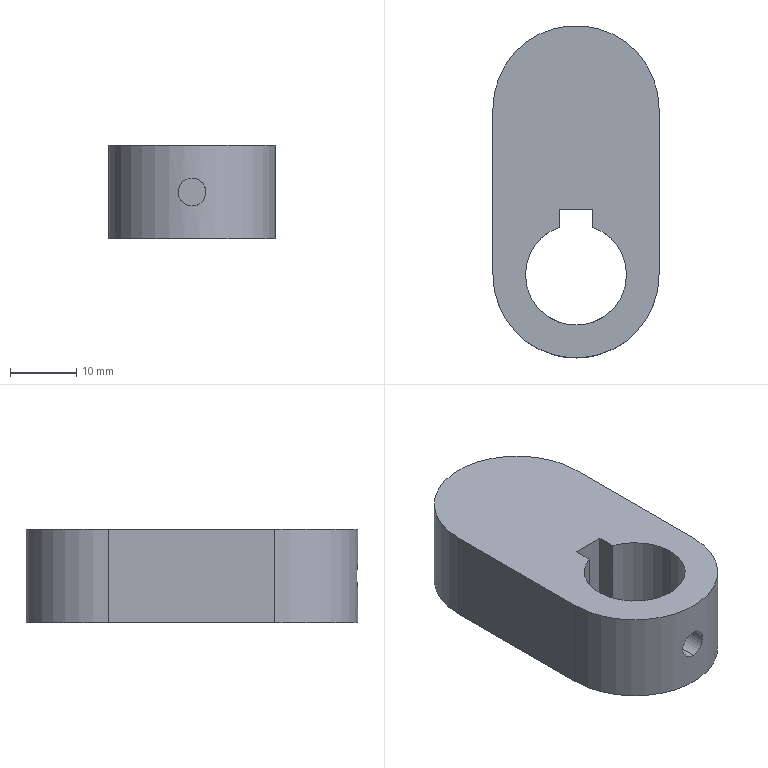Part | SolidWorks | features Extrusion 1, HoleWzd 1 | 1 solid | 14 faces | box 25 x 50 x 14 mm | volume 12843 mm3 | cylinder 7 | plane 7 | commonest cylinder face diameters 15.2 x3 4.2 x2 25 x2
STEP:
#1=CARTESIAN_POINT('',(0.,-12.5,4.9));
#2=VERTEX_POINT('',#1);
#3=CARTESIAN_POINT('',(0.,-12.5,9.1));
#4=VERTEX_POINT('',#3);
#5=CARTESIAN_POINT('',(0.,-12.5,4.9));
#6=CARTESIAN_POINT('',(-0.2743,-12.5,4.9));
#7=CARTESIAN_POINT('',(-0.5511,-12.49,4.955));
#8=CARTESIAN_POINT('',(-0.9302,-12.466,5.112));
#9=CARTESIAN_POINT('',(-1.053,-12.456,5.178));
#10=CARTESIAN_POINT('',(-1.282,-12.435,5.331));
#11=CARTESIAN_POINT('',(-1.387,-12.423,5.417));
#12=CARTESIAN_POINT('',(-1.581,-12.4,5.611));
#13=CARTESIAN_POINT('',(-1.669,-12.388,5.719));
#14=CARTESIAN_POINT('',(-1.822,-12.367,5.946));
#15=CARTESIAN_POINT('',(-1.886,-12.357,6.067));
#16=CARTESIAN_POINT('',(-1.992,-12.34,6.321));
#17=CARTESIAN_POINT('',(-2.032,-12.334,6.454));
#18=CARTESIAN_POINT('',(-2.086,-12.325,6.723));
#19=CARTESIAN_POINT('',(-2.1,-12.322,6.86));
#20=CARTESIAN_POINT('',(-2.1,-12.322,7.137));
#21=CARTESIAN_POINT('',(-2.087,-12.325,7.274));
#22=CARTESIAN_POINT('',(-2.033,-12.334,7.543));
#23=CARTESIAN_POINT('',(-1.993,-12.34,7.677));
#24=CARTESIAN_POINT('',(-1.888,-12.357,7.931));
#25=CARTESIAN_POINT('',(-1.823,-12.367,8.051));
#26=CARTESIAN_POINT('',(-1.671,-12.388,8.28));
#27=CARTESIAN_POINT('',(-1.582,-12.4,8.387));
#28=CARTESIAN_POINT('',(-1.293,-12.434,8.677));
#29=CARTESIAN_POINT('',(-1.059,-12.458,8.834));
#30=CARTESIAN_POINT('',(-0.6803,-12.482,8.991));
#31=CARTESIAN_POINT('',(-0.5475,-12.489,9.032));
#32=CARTESIAN_POINT('',(-0.2763,-12.498,9.086));
#33=CARTESIAN_POINT('',(-0.139,-12.5,9.1));
#34=CARTESIAN_POINT('',(0.,-12.5,9.1));
#35=B_SPLINE_CURVE_WITH_KNOTS('',3,(#5,#6,#7,#8,#9,#10,#11,#12,#13,#14,#15,#16,#17,#18,#19,#20,#21,#22,#23,#24,#25,#26,#27,#28,#29,#30,#31,#32,#33,#34),.UNSPECIFIED.,.F.,.F.,(4,2,2,2,2,2,2,2,2,2,2,2,2,2,4),(0.006577,0.007399,0.00781,0.008221,0.008632,0.009043,0.009454,0.009865,0.01028,0.01069,0.0111,0.01151,0.01233,0.01274,0.01315),.UNSPECIFIED.);
#36=EDGE_CURVE('',#2,#4,#35,.T.);
#37=ORIENTED_EDGE('',*,*,#36,.F.);
#38=CARTESIAN_POINT('',(0.,-7.6,4.9));
#39=VERTEX_POINT('',#38);
#40=CARTESIAN_POINT('',(0.,0.,4.9));
#41=DIRECTION('',(0.,1.,0.));
#42=VECTOR('',#41,1000.);
#43=LINE('',#40,#42);
#44=EDGE_CURVE('',#2,#39,#43,.T.);
#45=ORIENTED_EDGE('',*,*,#44,.T.);
#46=CARTESIAN_POINT('',(0.,-7.6,9.1));
#47=VERTEX_POINT('',#46);
#48=CARTESIAN_POINT('',(0.,-7.6,4.9));
#49=CARTESIAN_POINT('',(-0.2749,-7.6,4.9));
#50=CARTESIAN_POINT('',(-0.5524,-7.584,4.956));
#51=CARTESIAN_POINT('',(-0.932,-7.544,5.113));
#52=CARTESIAN_POINT('',(-1.055,-7.527,5.179));
#53=CARTESIAN_POINT('',(-1.282,-7.492,5.331));
#54=CARTESIAN_POINT('',(-1.388,-7.473,5.418));
#55=CARTESIAN_POINT('',(-1.581,-7.434,5.611));
#56=CARTESIAN_POINT('',(-1.669,-7.415,5.719));
#57=CARTESIAN_POINT('',(-1.821,-7.379,5.945));
#58=CARTESIAN_POINT('',(-1.886,-7.363,6.066));
#59=CARTESIAN_POINT('',(-1.992,-7.334,6.321));
#60=CARTESIAN_POINT('',(-2.032,-7.323,6.453));
#61=CARTESIAN_POINT('',(-2.086,-7.308,6.722));
#62=CARTESIAN_POINT('',(-2.1,-7.304,6.861));
#63=CARTESIAN_POINT('',(-2.1,-7.304,7.138));
#64=CARTESIAN_POINT('',(-2.086,-7.308,7.275));
#65=CARTESIAN_POINT('',(-2.033,-7.323,7.545));
#66=CARTESIAN_POINT('',(-1.992,-7.335,7.679));
#67=CARTESIAN_POINT('',(-1.834,-7.376,8.059));
#68=CARTESIAN_POINT('',(-1.678,-7.415,8.292));
#69=CARTESIAN_POINT('',(-1.389,-7.473,8.581));
#70=CARTESIAN_POINT('',(-1.283,-7.492,8.668));
#71=CARTESIAN_POINT('',(-1.054,-7.527,8.821));
#72=CARTESIAN_POINT('',(-0.9341,-7.543,8.886));
#73=CARTESIAN_POINT('',(-0.6811,-7.57,8.991));
#74=CARTESIAN_POINT('',(-0.5471,-7.581,9.032));
#75=CARTESIAN_POINT('',(-0.2767,-7.596,9.086));
#76=CARTESIAN_POINT('',(-0.1394,-7.6,9.1));
#77=CARTESIAN_POINT('',(0.,-7.6,9.1));
#78=B_SPLINE_CURVE_WITH_KNOTS('',3,(#48,#49,#50,#51,#52,#53,#54,#55,#56,#57,#58,#59,#60,#61,#62,#63,#64,#65,#66,#67,#68,#69,#70,#71,#72,#73,#74,#75,#76,#77),.UNSPECIFIED.,.F.,.F.,(4,2,2,2,2,2,2,2,2,2,2,2,2,2,4),(0.006598,0.007422,0.007835,0.008247,0.008659,0.009071,0.009484,0.009896,0.01031,0.01072,0.01154,0.01196,0.01237,0.01278,0.01319),.UNSPECIFIED.);
#79=EDGE_CURVE('',#39,#47,#78,.T.);
#80=ORIENTED_EDGE('',*,*,#79,.T.);
#81=CARTESIAN_POINT('',(0.,0.,9.1));
#82=DIRECTION('',(0.,1.,0.));
#83=VECTOR('',#82,1000.);
#84=LINE('',#81,#83);
#85=EDGE_CURVE('',#4,#47,#84,.T.);
#86=ORIENTED_EDGE('',*,*,#85,.F.);
#87=EDGE_LOOP('',(#37,#45,#80,#86));
#88=FACE_OUTER_BOUND('',#87,.T.);
#89=CARTESIAN_POINT('',(0.,0.,7.));
#90=DIRECTION('',(0.,1.,0.));
#91=DIRECTION('',(0.,0.,1.));
#92=AXIS2_PLACEMENT_3D('',#89,#90,#91);
#93=CYLINDRICAL_SURFACE('',#92,2.1);
#94=ADVANCED_FACE('',(#88),#93,.F.);
#95=CARTESIAN_POINT('',(0.,-7.6,9.1));
#96=CARTESIAN_POINT('',(0.1395,-7.6,9.1));
#97=CARTESIAN_POINT('',(0.2765,-7.596,9.086));
#98=CARTESIAN_POINT('',(0.5459,-7.582,9.032));
#99=CARTESIAN_POINT('',(0.6796,-7.571,8.992));
#100=CARTESIAN_POINT('',(0.9337,-7.544,8.886));
#101=CARTESIAN_POINT('',(1.054,-7.527,8.821));
#102=CARTESIAN_POINT('',(1.282,-7.492,8.669));
#103=CARTESIAN_POINT('',(1.389,-7.473,8.581));
#104=CARTESIAN_POINT('',(1.678,-7.415,8.292));
#105=CARTESIAN_POINT('',(1.834,-7.376,8.058));
#106=CARTESIAN_POINT('',(1.992,-7.335,7.68));
#107=CARTESIAN_POINT('',(2.032,-7.323,7.547));
#108=CARTESIAN_POINT('',(2.086,-7.308,7.275));
#109=CARTESIAN_POINT('',(2.1,-7.304,7.139));
#110=CARTESIAN_POINT('',(2.1,-7.304,6.863));
#111=CARTESIAN_POINT('',(2.086,-7.308,6.723));
#112=CARTESIAN_POINT('',(2.032,-7.323,6.453));
#113=CARTESIAN_POINT('',(1.992,-7.334,6.322));
#114=CARTESIAN_POINT('',(1.833,-7.376,5.939));
#115=CARTESIAN_POINT('',(1.679,-7.415,5.709));
#116=CARTESIAN_POINT('',(1.387,-7.473,5.418));
#117=CARTESIAN_POINT('',(1.282,-7.492,5.331));
#118=CARTESIAN_POINT('',(1.055,-7.527,5.179));
#119=CARTESIAN_POINT('',(0.9321,-7.544,5.113));
#120=CARTESIAN_POINT('',(0.6787,-7.571,5.008));
#121=CARTESIAN_POINT('',(0.5477,-7.581,4.968));
#122=CARTESIAN_POINT('',(0.2769,-7.596,4.914));
#123=CARTESIAN_POINT('',(0.1375,-7.6,4.9));
#124=CARTESIAN_POINT('',(0.,-7.6,4.9));
#125=B_SPLINE_CURVE_WITH_KNOTS('',3,(#95,#96,#97,#98,#99,#100,#101,#102,#103,#104,#105,#106,#107,#108,#109,#110,#111,#112,#113,#114,#115,#116,#117,#118,#119,#120,#121,#122,#123,#124),.UNSPECIFIED.,.F.,.F.,(4,2,2,2,2,2,2,2,2,2,2,2,2,2,4),(0.,0.0004124,0.0008247,0.001237,0.001649,0.002474,0.002887,0.003299,0.003711,0.004124,0.004948,0.005361,0.005773,0.006185,0.006598),.UNSPECIFIED.);
#126=EDGE_CURVE('',#47,#39,#125,.T.);
#127=ORIENTED_EDGE('',*,*,#126,.F.);
#128=ORIENTED_EDGE('',*,*,#79,.F.);
#129=EDGE_LOOP('',(#127,#128));
#130=FACE_BOUND('',#129,.T.);
#131=CARTESIAN_POINT('',(-7.6,0.,14.));
#132=VERTEX_POINT('',#131);
#133=CARTESIAN_POINT('',(7.6,0.,14.));
#134=VERTEX_POINT('',#133);
#135=CARTESIAN_POINT('',(0.,0.,14.));
#136=DIRECTION('',(0.,0.,1.));
#137=DIRECTION('',(1.,0.,0.));
#138=AXIS2_PLACEMENT_3D('',#135,#136,#137);
#139=CIRCLE('',#138,7.6);
#140=EDGE_CURVE('',#132,#134,#139,.T.);
#141=ORIENTED_EDGE('',*,*,#140,.T.);
#142=CARTESIAN_POINT('',(7.6,0.,0.));
#143=VERTEX_POINT('',#142);
#144=CARTESIAN_POINT('',(7.6,0.,14.));
#145=DIRECTION('',(0.,0.,-1.));
#146=VECTOR('',#145,1000.);
#147=LINE('',#144,#146);
#148=EDGE_CURVE('',#134,#143,#147,.T.);
#149=ORIENTED_EDGE('',*,*,#148,.T.);
#150=CARTESIAN_POINT('',(-7.6,0.,0.));
#151=VERTEX_POINT('',#150);
#152=CARTESIAN_POINT('',(0.,0.,0.));
#153=DIRECTION('',(0.,0.,1.));
#154=DIRECTION('',(1.,0.,0.));
#155=AXIS2_PLACEMENT_3D('',#152,#153,#154);
#156=CIRCLE('',#155,7.6);
#157=EDGE_CURVE('',#151,#143,#156,.T.);
#158=ORIENTED_EDGE('',*,*,#157,.F.);
#159=CARTESIAN_POINT('',(-7.6,0.,14.));
#160=DIRECTION('',(0.,0.,-1.));
#161=VECTOR('',#160,1000.);
#162=LINE('',#159,#161);
#163=EDGE_CURVE('',#132,#151,#162,.T.);
#164=ORIENTED_EDGE('',*,*,#163,.F.);
#165=EDGE_LOOP('',(#141,#149,#158,#164));
#166=FACE_OUTER_BOUND('',#165,.T.);
#167=CARTESIAN_POINT('',(0.,0.,14.));
#168=DIRECTION('',(0.,0.,-1.));
#169=DIRECTION('',(-1.,0.,0.));
#170=AXIS2_PLACEMENT_3D('',#167,#168,#169);
#171=CYLINDRICAL_SURFACE('',#170,7.6);
#172=ADVANCED_FACE('',(#130,#166),#171,.F.);
#173=CARTESIAN_POINT('',(-2.5,7.177,14.));
#174=VERTEX_POINT('',#173);
#175=CARTESIAN_POINT('',(0.,0.,14.));
#176=DIRECTION('',(0.,0.,1.));
#177=DIRECTION('',(1.,0.,0.));
#178=AXIS2_PLACEMENT_3D('',#175,#176,#177);
#179=CIRCLE('',#178,7.6);
#180=EDGE_CURVE('',#174,#132,#179,.T.);
#181=ORIENTED_EDGE('',*,*,#180,.T.);
#182=ORIENTED_EDGE('',*,*,#163,.T.);
#183=CARTESIAN_POINT('',(-2.5,7.177,0.));
#184=VERTEX_POINT('',#183);
#185=CARTESIAN_POINT('',(0.,0.,0.));
#186=DIRECTION('',(0.,0.,1.));
#187=DIRECTION('',(1.,0.,0.));
#188=AXIS2_PLACEMENT_3D('',#185,#186,#187);
#189=CIRCLE('',#188,7.6);
#190=EDGE_CURVE('',#184,#151,#189,.T.);
#191=ORIENTED_EDGE('',*,*,#190,.F.);
#192=CARTESIAN_POINT('',(-2.5,7.177,14.));
#193=DIRECTION('',(0.,0.,-1.));
#194=VECTOR('',#193,1000.);
#195=LINE('',#192,#194);
#196=EDGE_CURVE('',#174,#184,#195,.T.);
#197=ORIENTED_EDGE('',*,*,#196,.F.);
#198=EDGE_LOOP('',(#181,#182,#191,#197));
#199=FACE_OUTER_BOUND('',#198,.T.);
#200=CARTESIAN_POINT('',(0.,0.,14.));
#201=DIRECTION('',(0.,0.,-1.));
#202=DIRECTION('',(-1.,0.,0.));
#203=AXIS2_PLACEMENT_3D('',#200,#201,#202);
#204=CYLINDRICAL_SURFACE('',#203,7.6);
#205=ADVANCED_FACE('',(#199),#204,.F.);
#206=CARTESIAN_POINT('',(12.5,0.,0.));
#207=VERTEX_POINT('',#206);
#208=CARTESIAN_POINT('',(12.5,25.,0.));
#209=VERTEX_POINT('',#208);
#210=CARTESIAN_POINT('',(12.5,0.,0.));
#211=DIRECTION('',(0.,1.,0.));
#212=VECTOR('',#211,1000.);
#213=LINE('',#210,#212);
#214=EDGE_CURVE('',#207,#209,#213,.T.);
#215=ORIENTED_EDGE('',*,*,#214,.T.);
#216=CARTESIAN_POINT('',(12.5,25.,14.));
#217=VERTEX_POINT('',#216);
#218=CARTESIAN_POINT('',(12.5,25.,14.));
#219=DIRECTION('',(0.,0.,-1.));
#220=VECTOR('',#219,1000.);
#221=LINE('',#218,#220);
#222=EDGE_CURVE('',#217,#209,#221,.T.);
#223=ORIENTED_EDGE('',*,*,#222,.F.);
#224=CARTESIAN_POINT('',(12.5,0.,14.));
#225=VERTEX_POINT('',#224);
#226=CARTESIAN_POINT('',(12.5,0.,14.));
#227=DIRECTION('',(0.,1.,0.));
#228=VECTOR('',#227,1000.);
#229=LINE('',#226,#228);
#230=EDGE_CURVE('',#225,#217,#229,.T.);
#231=ORIENTED_EDGE('',*,*,#230,.F.);
#232=CARTESIAN_POINT('',(12.5,0.,14.));
#233=DIRECTION('',(0.,0.,-1.));
#234=VECTOR('',#233,1000.);
#235=LINE('',#232,#234);
#236=EDGE_CURVE('',#225,#207,#235,.T.);
#237=ORIENTED_EDGE('',*,*,#236,.T.);
#238=EDGE_LOOP('',(#215,#223,#231,#237));
#239=FACE_OUTER_BOUND('',#238,.T.);
#240=CARTESIAN_POINT('',(12.5,0.,14.));
#241=DIRECTION('',(-1.,0.,0.));
#242=DIRECTION('',(0.,0.,1.));
#243=AXIS2_PLACEMENT_3D('',#240,#241,#242);
#244=PLANE('',#243);
#245=ADVANCED_FACE('',(#239),#244,.F.);
#246=CARTESIAN_POINT('',(-12.5,25.,0.));
#247=VERTEX_POINT('',#246);
#248=CARTESIAN_POINT('',(0.,25.,0.));
#249=DIRECTION('',(0.,0.,1.));
#250=DIRECTION('',(1.,0.,0.));
#251=AXIS2_PLACEMENT_3D('',#248,#249,#250);
#252=CIRCLE('',#251,12.5);
#253=EDGE_CURVE('',#209,#247,#252,.T.);
#254=ORIENTED_EDGE('',*,*,#253,.T.);
#255=CARTESIAN_POINT('',(-12.5,25.,14.));
#256=VERTEX_POINT('',#255);
#257=CARTESIAN_POINT('',(-12.5,25.,14.));
#258=DIRECTION('',(0.,0.,-1.));
#259=VECTOR('',#258,1000.);
#260=LINE('',#257,#259);
#261=EDGE_CURVE('',#256,#247,#260,.T.);
#262=ORIENTED_EDGE('',*,*,#261,.F.);
#263=CARTESIAN_POINT('',(0.,25.,14.));
#264=DIRECTION('',(0.,0.,1.));
#265=DIRECTION('',(1.,0.,0.));
#266=AXIS2_PLACEMENT_3D('',#263,#264,#265);
#267=CIRCLE('',#266,12.5);
#268=EDGE_CURVE('',#217,#256,#267,.T.);
#269=ORIENTED_EDGE('',*,*,#268,.F.);
#270=ORIENTED_EDGE('',*,*,#222,.T.);
#271=EDGE_LOOP('',(#254,#262,#269,#270));
#272=FACE_OUTER_BOUND('',#271,.T.);
#273=CARTESIAN_POINT('',(0.,25.,14.));
#274=DIRECTION('',(0.,0.,-1.));
#275=DIRECTION('',(-1.,0.,0.));
#276=AXIS2_PLACEMENT_3D('',#273,#274,#275);
#277=CYLINDRICAL_SURFACE('',#276,12.5);
#278=ADVANCED_FACE('',(#272),#277,.T.);
#279=CARTESIAN_POINT('',(-12.5,0.,0.));
#280=VERTEX_POINT('',#279);
#281=CARTESIAN_POINT('',(-12.5,0.,0.));
#282=DIRECTION('',(0.,1.,0.));
#283=VECTOR('',#282,1000.);
#284=LINE('',#281,#283);
#285=EDGE_CURVE('',#280,#247,#284,.T.);
#286=ORIENTED_EDGE('',*,*,#285,.F.);
#287=CARTESIAN_POINT('',(-12.5,0.,14.));
#288=VERTEX_POINT('',#287);
#289=CARTESIAN_POINT('',(-12.5,0.,14.));
#290=DIRECTION('',(0.,0.,-1.));
#291=VECTOR('',#290,1000.);
#292=LINE('',#289,#291);
#293=EDGE_CURVE('',#288,#280,#292,.T.);
#294=ORIENTED_EDGE('',*,*,#293,.F.);
#295=CARTESIAN_POINT('',(-12.5,0.,14.));
#296=DIRECTION('',(0.,1.,0.));
#297=VECTOR('',#296,1000.);
#298=LINE('',#295,#297);
#299=EDGE_CURVE('',#288,#256,#298,.T.);
#300=ORIENTED_EDGE('',*,*,#299,.T.);
#301=ORIENTED_EDGE('',*,*,#261,.T.);
#302=EDGE_LOOP('',(#286,#294,#300,#301));
#303=FACE_OUTER_BOUND('',#302,.T.);
#304=CARTESIAN_POINT('',(-12.5,0.,14.));
#305=DIRECTION('',(-1.,0.,0.));
#306=DIRECTION('',(0.,0.,1.));
#307=AXIS2_PLACEMENT_3D('',#304,#305,#306);
#308=PLANE('',#307);
#309=ADVANCED_FACE('',(#303),#308,.T.);
#310=ORIENTED_EDGE('',*,*,#148,.F.);
#311=CARTESIAN_POINT('',(2.5,7.177,14.));
#312=VERTEX_POINT('',#311);
#313=CARTESIAN_POINT('',(0.,0.,14.));
#314=DIRECTION('',(0.,0.,1.));
#315=DIRECTION('',(1.,0.,0.));
#316=AXIS2_PLACEMENT_3D('',#313,#314,#315);
#317=CIRCLE('',#316,7.6);
#318=EDGE_CURVE('',#134,#312,#317,.T.);
#319=ORIENTED_EDGE('',*,*,#318,.T.);
#320=CARTESIAN_POINT('',(2.5,7.177,0.));
#321=VERTEX_POINT('',#320);
#322=CARTESIAN_POINT('',(2.5,7.177,14.));
#323=DIRECTION('',(0.,0.,-1.));
#324=VECTOR('',#323,1000.);
#325=LINE('',#322,#324);
#326=EDGE_CURVE('',#312,#321,#325,.T.);
#327=ORIENTED_EDGE('',*,*,#326,.T.);
#328=CARTESIAN_POINT('',(0.,0.,0.));
#329=DIRECTION('',(0.,0.,1.));
#330=DIRECTION('',(1.,0.,0.));
#331=AXIS2_PLACEMENT_3D('',#328,#329,#330);
#332=CIRCLE('',#331,7.6);
#333=EDGE_CURVE('',#143,#321,#332,.T.);
#334=ORIENTED_EDGE('',*,*,#333,.F.);
#335=EDGE_LOOP('',(#310,#319,#327,#334));
#336=FACE_OUTER_BOUND('',#335,.T.);
#337=CARTESIAN_POINT('',(0.,0.,14.));
#338=DIRECTION('',(0.,0.,-1.));
#339=DIRECTION('',(-1.,0.,0.));
#340=AXIS2_PLACEMENT_3D('',#337,#338,#339);
#341=CYLINDRICAL_SURFACE('',#340,7.6);
#342=ADVANCED_FACE('',(#336),#341,.F.);
#343=CARTESIAN_POINT('',(-2.5,9.9,0.));
#344=VERTEX_POINT('',#343);
#345=CARTESIAN_POINT('',(-2.5,0.,0.));
#346=DIRECTION('',(0.,1.,0.));
#347=VECTOR('',#346,1000.);
#348=LINE('',#345,#347);
#349=EDGE_CURVE('',#184,#344,#348,.T.);
#350=ORIENTED_EDGE('',*,*,#349,.T.);
#351=CARTESIAN_POINT('',(-2.5,9.9,14.));
#352=VERTEX_POINT('',#351);
#353=CARTESIAN_POINT('',(-2.5,9.9,14.));
#354=DIRECTION('',(0.,0.,-1.));
#355=VECTOR('',#354,1000.);
#356=LINE('',#353,#355);
#357=EDGE_CURVE('',#352,#344,#356,.T.);
#358=ORIENTED_EDGE('',*,*,#357,.F.);
#359=CARTESIAN_POINT('',(-2.5,0.,14.));
#360=DIRECTION('',(0.,1.,0.));
#361=VECTOR('',#360,1000.);
#362=LINE('',#359,#361);
#363=EDGE_CURVE('',#174,#352,#362,.T.);
#364=ORIENTED_EDGE('',*,*,#363,.F.);
#365=ORIENTED_EDGE('',*,*,#196,.T.);
#366=EDGE_LOOP('',(#350,#358,#364,#365));
#367=FACE_OUTER_BOUND('',#366,.T.);
#368=CARTESIAN_POINT('',(-2.5,0.,14.));
#369=DIRECTION('',(-1.,0.,0.));
#370=DIRECTION('',(0.,0.,1.));
#371=AXIS2_PLACEMENT_3D('',#368,#369,#370);
#372=PLANE('',#371);
#373=ADVANCED_FACE('',(#367),#372,.F.);
#374=CARTESIAN_POINT('',(2.5,9.9,0.));
#375=VERTEX_POINT('',#374);
#376=CARTESIAN_POINT('',(0.,9.9,0.));
#377=DIRECTION('',(-1.,0.,0.));
#378=VECTOR('',#377,1000.);
#379=LINE('',#376,#378);
#380=EDGE_CURVE('',#375,#344,#379,.T.);
#381=ORIENTED_EDGE('',*,*,#380,.F.);
#382=CARTESIAN_POINT('',(2.5,9.9,14.));
#383=VERTEX_POINT('',#382);
#384=CARTESIAN_POINT('',(2.5,9.9,14.));
#385=DIRECTION('',(0.,0.,-1.));
#386=VECTOR('',#385,1000.);
#387=LINE('',#384,#386);
#388=EDGE_CURVE('',#383,#375,#387,.T.);
#389=ORIENTED_EDGE('',*,*,#388,.F.);
#390=CARTESIAN_POINT('',(0.,9.9,14.));
#391=DIRECTION('',(-1.,0.,0.));
#392=VECTOR('',#391,1000.);
#393=LINE('',#390,#392);
#394=EDGE_CURVE('',#383,#352,#393,.T.);
#395=ORIENTED_EDGE('',*,*,#394,.T.);
#396=ORIENTED_EDGE('',*,*,#357,.T.);
#397=EDGE_LOOP('',(#381,#389,#395,#396));
#398=FACE_OUTER_BOUND('',#397,.T.);
#399=CARTESIAN_POINT('',(0.,9.9,14.));
#400=DIRECTION('',(0.,-1.,0.));
#401=DIRECTION('',(0.,0.,-1.));
#402=AXIS2_PLACEMENT_3D('',#399,#400,#401);
#403=PLANE('',#402);
#404=ADVANCED_FACE('',(#398),#403,.T.);
#405=CARTESIAN_POINT('',(2.5,0.,0.));
#406=DIRECTION('',(0.,1.,0.));
#407=VECTOR('',#406,1000.);
#408=LINE('',#405,#407);
#409=EDGE_CURVE('',#321,#375,#408,.T.);
#410=ORIENTED_EDGE('',*,*,#409,.F.);
#411=ORIENTED_EDGE('',*,*,#326,.F.);
#412=CARTESIAN_POINT('',(2.5,0.,14.));
#413=DIRECTION('',(0.,1.,0.));
#414=VECTOR('',#413,1000.);
#415=LINE('',#412,#414);
#416=EDGE_CURVE('',#312,#383,#415,.T.);
#417=ORIENTED_EDGE('',*,*,#416,.T.);
#418=ORIENTED_EDGE('',*,*,#388,.T.);
#419=EDGE_LOOP('',(#410,#411,#417,#418));
#420=FACE_OUTER_BOUND('',#419,.T.);
#421=CARTESIAN_POINT('',(2.5,0.,14.));
#422=DIRECTION('',(-1.,0.,0.));
#423=DIRECTION('',(0.,0.,1.));
#424=AXIS2_PLACEMENT_3D('',#421,#422,#423);
#425=PLANE('',#424);
#426=ADVANCED_FACE('',(#420),#425,.T.);
#427=CARTESIAN_POINT('',(0.,-12.5,9.1));
#428=CARTESIAN_POINT('',(0.139,-12.5,9.1));
#429=CARTESIAN_POINT('',(0.2757,-12.498,9.086));
#430=CARTESIAN_POINT('',(0.5444,-12.489,9.033));
#431=CARTESIAN_POINT('',(0.6779,-12.482,8.992));
#432=CARTESIAN_POINT('',(0.9322,-12.466,8.887));
#433=CARTESIAN_POINT('',(1.053,-12.456,8.822));
#434=CARTESIAN_POINT('',(1.281,-12.435,8.67));
#435=CARTESIAN_POINT('',(1.389,-12.423,8.581));
#436=CARTESIAN_POINT('',(1.679,-12.388,8.291));
#437=CARTESIAN_POINT('',(1.835,-12.365,8.057));
#438=CARTESIAN_POINT('',(2.045,-12.332,7.552));
#439=CARTESIAN_POINT('',(2.1,-12.322,7.275));
#440=CARTESIAN_POINT('',(2.1,-12.322,6.864));
#441=CARTESIAN_POINT('',(2.086,-12.325,6.724));
#442=CARTESIAN_POINT('',(2.033,-12.334,6.455));
#443=CARTESIAN_POINT('',(1.993,-12.34,6.324));
#444=CARTESIAN_POINT('',(1.887,-12.357,6.069));
#445=CARTESIAN_POINT('',(1.822,-12.367,5.946));
#446=CARTESIAN_POINT('',(1.67,-12.388,5.719));
#447=CARTESIAN_POINT('',(1.583,-12.4,5.613));
#448=CARTESIAN_POINT('',(1.387,-12.423,5.417));
#449=CARTESIAN_POINT('',(1.281,-12.435,5.331));
#450=CARTESIAN_POINT('',(1.054,-12.456,5.179));
#451=CARTESIAN_POINT('',(0.9312,-12.466,5.113));
#452=CARTESIAN_POINT('',(0.6771,-12.482,5.007));
#453=CARTESIAN_POINT('',(0.5462,-12.489,4.968));
#454=CARTESIAN_POINT('',(0.2765,-12.498,4.914));
#455=CARTESIAN_POINT('',(0.1372,-12.5,4.9));
#456=CARTESIAN_POINT('',(0.,-12.5,4.9));
#457=B_SPLINE_CURVE_WITH_KNOTS('',3,(#427,#428,#429,#430,#431,#432,#433,#434,#435,#436,#437,#438,#439,#440,#441,#442,#443,#444,#445,#446,#447,#448,#449,#450,#451,#452,#453,#454,#455,#456),.UNSPECIFIED.,.F.,.F.,(4,2,2,2,2,2,2,2,2,2,2,2,2,2,4),(0.,0.0004111,0.0008222,0.001233,0.001644,0.002466,0.003289,0.0037,0.004111,0.004522,0.004933,0.005344,0.005755,0.006166,0.006577),.UNSPECIFIED.);
#458=EDGE_CURVE('',#4,#2,#457,.T.);
#459=ORIENTED_EDGE('',*,*,#458,.T.);
#460=ORIENTED_EDGE('',*,*,#36,.T.);
#461=EDGE_LOOP('',(#459,#460));
#462=FACE_BOUND('',#461,.T.);
#463=CARTESIAN_POINT('',(0.,0.,0.));
#464=DIRECTION('',(0.,0.,1.));
#465=DIRECTION('',(1.,0.,0.));
#466=AXIS2_PLACEMENT_3D('',#463,#464,#465);
#467=CIRCLE('',#466,12.5);
#468=EDGE_CURVE('',#280,#207,#467,.T.);
#469=ORIENTED_EDGE('',*,*,#468,.T.);
#470=ORIENTED_EDGE('',*,*,#236,.F.);
#471=CARTESIAN_POINT('',(0.,0.,14.));
#472=DIRECTION('',(0.,0.,1.));
#473=DIRECTION('',(1.,0.,0.));
#474=AXIS2_PLACEMENT_3D('',#471,#472,#473);
#475=CIRCLE('',#474,12.5);
#476=EDGE_CURVE('',#288,#225,#475,.T.);
#477=ORIENTED_EDGE('',*,*,#476,.F.);
#478=ORIENTED_EDGE('',*,*,#293,.T.);
#479=EDGE_LOOP('',(#469,#470,#477,#478));
#480=FACE_OUTER_BOUND('',#479,.T.);
#481=CARTESIAN_POINT('',(0.,0.,14.));
#482=DIRECTION('',(0.,0.,-1.));
#483=DIRECTION('',(-1.,0.,0.));
#484=AXIS2_PLACEMENT_3D('',#481,#482,#483);
#485=CYLINDRICAL_SURFACE('',#484,12.5);
#486=ADVANCED_FACE('',(#462,#480),#485,.T.);
#487=ORIENTED_EDGE('',*,*,#180,.F.);
#488=ORIENTED_EDGE('',*,*,#363,.T.);
#489=ORIENTED_EDGE('',*,*,#394,.F.);
#490=ORIENTED_EDGE('',*,*,#416,.F.);
#491=ORIENTED_EDGE('',*,*,#318,.F.);
#492=ORIENTED_EDGE('',*,*,#140,.F.);
#493=EDGE_LOOP('',(#487,#488,#489,#490,#491,#492));
#494=FACE_BOUND('',#493,.T.);
#495=ORIENTED_EDGE('',*,*,#230,.T.);
#496=ORIENTED_EDGE('',*,*,#268,.T.);
#497=ORIENTED_EDGE('',*,*,#299,.F.);
#498=ORIENTED_EDGE('',*,*,#476,.T.);
#499=EDGE_LOOP('',(#495,#496,#497,#498));
#500=FACE_OUTER_BOUND('',#499,.T.);
#501=CARTESIAN_POINT('',(0.,0.,14.));
#502=DIRECTION('',(0.,0.,1.));
#503=DIRECTION('',(1.,0.,0.));
#504=AXIS2_PLACEMENT_3D('',#501,#502,#503);
#505=PLANE('',#504);
#506=ADVANCED_FACE('',(#494,#500),#505,.T.);
#507=ORIENTED_EDGE('',*,*,#190,.T.);
#508=ORIENTED_EDGE('',*,*,#157,.T.);
#509=ORIENTED_EDGE('',*,*,#333,.T.);
#510=ORIENTED_EDGE('',*,*,#409,.T.);
#511=ORIENTED_EDGE('',*,*,#380,.T.);
#512=ORIENTED_EDGE('',*,*,#349,.F.);
#513=EDGE_LOOP('',(#507,#508,#509,#510,#511,#512));
#514=FACE_BOUND('',#513,.T.);
#515=ORIENTED_EDGE('',*,*,#214,.F.);
#516=ORIENTED_EDGE('',*,*,#468,.F.);
#517=ORIENTED_EDGE('',*,*,#285,.T.);
#518=ORIENTED_EDGE('',*,*,#253,.F.);
#519=EDGE_LOOP('',(#515,#516,#517,#518));
#520=FACE_OUTER_BOUND('',#519,.T.);
#521=CARTESIAN_POINT('',(0.,0.,0.));
#522=DIRECTION('',(0.,0.,1.));
#523=DIRECTION('',(1.,0.,0.));
#524=AXIS2_PLACEMENT_3D('',#521,#522,#523);
#525=PLANE('',#524);
#526=ADVANCED_FACE('',(#514,#520),#525,.F.);
#527=ORIENTED_EDGE('',*,*,#44,.F.);
#528=ORIENTED_EDGE('',*,*,#458,.F.);
#529=ORIENTED_EDGE('',*,*,#85,.T.);
#530=ORIENTED_EDGE('',*,*,#126,.T.);
#531=EDGE_LOOP('',(#527,#528,#529,#530));
#532=FACE_OUTER_BOUND('',#531,.T.);
#533=CARTESIAN_POINT('',(0.,0.,7.));
#534=DIRECTION('',(0.,1.,0.));
#535=DIRECTION('',(0.,0.,1.));
#536=AXIS2_PLACEMENT_3D('',#533,#534,#535);
#537=CYLINDRICAL_SURFACE('',#536,2.1);
#538=ADVANCED_FACE('',(#532),#537,.F.);
#539=CLOSED_SHELL('',(#94,#172,#205,#245,#278,#309,#342,#373,#404,#426,#486,#506,#526,#538));
#540=MANIFOLD_SOLID_BREP('',#539);
#541=CARTESIAN_POINT('',(0.,0.,0.));
#542=DIRECTION('',(0.,0.,1.));
#543=DIRECTION('',(1.,0.,0.));
#544=AXIS2_PLACEMENT_3D('',#541,#542,#543);
#545=(LENGTH_UNIT()NAMED_UNIT(*)SI_UNIT(.MILLI.,.METRE.));
#546=UNCERTAINTY_MEASURE_WITH_UNIT(LENGTH_MEASURE(0.00001),#545,'','');
#547=(NAMED_UNIT(*)PLANE_ANGLE_UNIT()SI_UNIT($,.RADIAN.));
#548=(NAMED_UNIT(*)SI_UNIT($,.STERADIAN.)SOLID_ANGLE_UNIT());
#549=(GEOMETRIC_REPRESENTATION_CONTEXT(3)GLOBAL_UNCERTAINTY_ASSIGNED_CONTEXT((#546))GLOBAL_UNIT_ASSIGNED_CONTEXT((#545,#547,#548))REPRESENTATION_CONTEXT('',''));
#550=ADVANCED_BREP_SHAPE_REPRESENTATION('',(#540,#544),#549);